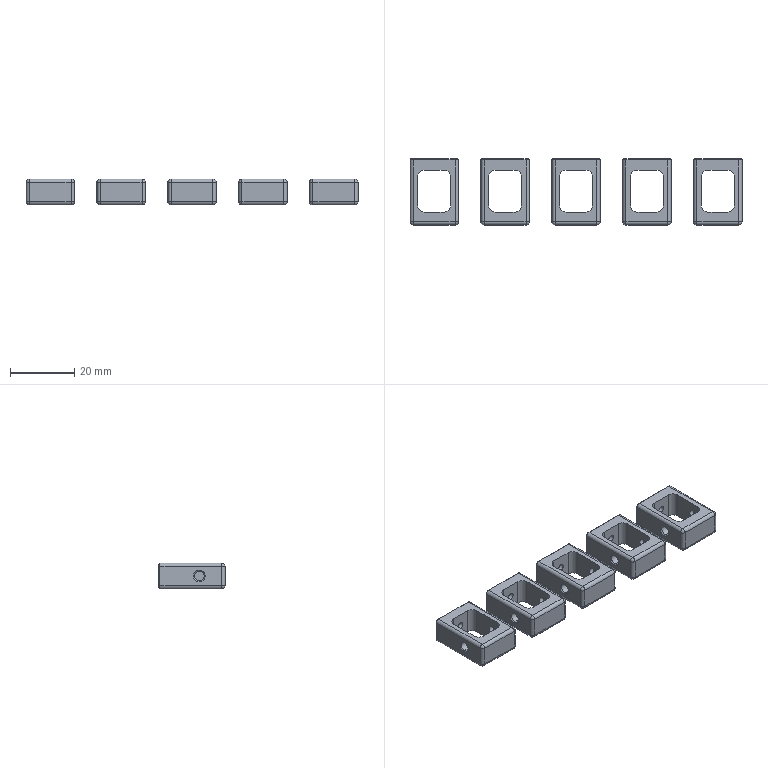NC program | NX | posted with a generic post | part box 103 x 20.5 x 8 mm
Lines 8374 to 9732 of 9732:
(PLANAR_MILL_COPY , TOOL : D6A45)
N16728 T01 M6
N16730 G54
N16732 G17 G0 G90 X-47. Y1.52 S9500 M3
N16734 G43 Z30. H1
N16736 Z0.5
N16738 G94 G1 Z-1. F1250.
N16740 X-47.7 Y1.116
N16742 G3 X-48.2 Y0.25 R1.
N16744 G1 Y-4.25
N16746 G3 X-47.1 Y-5.35 R1.1
N16748 G1 X-40.9
N16750 G3 X-39.8 Y-4.25 R1.1
N16752 G1 Y4.75
N16754 G3 X-40.9 Y5.85 R1.1
N16756 G1 X-47.1
N16758 G3 X-48.2 Y4.75 R1.1
N16760 G1 Y0.25
N16762 G3 X-47.7 Y-0.616 R1.
N16764 G1 X-47. Y-1.02
N16766 Z0.5
N16768 G0 Z30.
N16770 X-25. Y1.52
N16772 Z0.5
N16774 G1 Z-1.
N16776 X-25.7 Y1.116
N16778 G3 X-26.2 Y0.25 R1.
N16780 G1 Y-4.25
N16782 G3 X-25.1 Y-5.35 R1.1
N16784 G1 X-18.9
N16786 G3 X-17.8 Y-4.25 R1.1
N16788 G1 Y4.75
N16790 G3 X-18.9 Y5.85 R1.1
N16792 G1 X-25.1
N16794 G3 X-26.2 Y4.75 R1.1
N16796 G1 Y0.25
N16798 G3 X-25.7 Y-0.616 R1.
N16800 G1 X-25. Y-1.02
N16802 Z0.5
N16804 G0 Z30.
N16806 X-3. Y1.52
N16808 Z0.5
N16810 G1 Z-1.
N16812 X-3.7 Y1.116
N16814 G3 X-4.2 Y0.25 R1.
N16816 G1 Y-4.25
N16818 G3 X-3.1 Y-5.35 R1.1
N16820 G1 X3.1
N16822 G3 X4.2 Y-4.25 R1.1
N16824 G1 Y4.75
N16826 G3 X3.1 Y5.85 R1.1
N16828 G1 X-3.1
N16830 G3 X-4.2 Y4.75 R1.1
N16832 G1 Y0.25
N16834 G3 X-3.7 Y-0.616 R1.
N16836 G1 X-3. Y-1.02
N16838 Z0.5
N16840 G0 Z30.
N16842 X19. Y1.52
N16844 Z0.5
N16846 G1 Z-1.
N16848 X18.3 Y1.116
N16850 G3 X17.8 Y0.25 R1.
N16852 G1 Y-4.25
N16854 G3 X18.9 Y-5.35 R1.1
N16856 G1 X25.1
N16858 G3 X26.2 Y-4.25 R1.1
N16860 G1 Y4.75
N16862 G3 X25.1 Y5.85 R1.1
N16864 G1 X18.9
N16866 G3 X17.8 Y4.75 R1.1
N16868 G1 Y0.25
N16870 G3 X18.3 Y-0.616 R1.
N16872 G1 X19. Y-1.02
N16874 Z0.5
N16876 G0 Z30.
N16878 X47.
N16880 Z0.5
N16882 G1 Z-1.
N16884 X47.7 Y-0.616
N16886 G3 X48.2 Y0.25 R1.
N16888 G1 Y4.75
N16890 G3 X47.1 Y5.85 R1.1
N16892 G1 X40.9
N16894 G3 X39.8 Y4.75 R1.1
N16896 G1 Y-4.25
N16898 G3 X40.9 Y-5.35 R1.1
N16900 G1 X47.1
N16902 G3 X48.2 Y-4.25 R1.1
N16904 G1 Y0.25
N16906 G3 X47.7 Y1.116 R1.
N16908 G1 X47. Y1.52
N16910 Z0.5
N16912 G0 Z30.
N16914 M5
(ZLEVEL_PROFILE_1 , TOOL : D4R0.5)
N16916 T16 M6
N16918 G54
N16920 G17 G0 G90 X-35.174 Y12.738 S9500 M3
N16922 G43 Z30. H16
N16924 Z1.488
N16926 G94 G1 Z-0.012 F3000.
N16928 X-35.682 Y12.485
N16930 G3 X-35.903 Y12.152 R0.4
N16932 X-35.813 Y9.95 R10.813
N16934 G1 Y-9.25
N16936 G2 X-37.5 Y-10.937 R1.687
N16938 G1 X-50.5
N16940 G2 X-52.187 Y-9.25 R1.687
N16942 G1 Y9.95
N16944 X-52.109 Y10.153
N16946 X-52.09 Y12.155
N16948 X-52.133 Y12.154 Z-0.018
N16950 X-52.161 Y12.153 Z-0.024
N16952 X-52.25 Y10.153
N16954 X-52.27 Y9.95
N16956 Y-9.25
N16958 G3 X-50.5 Y-11.02 R1.77
N16960 G1 X-37.5
N16962 G3 X-35.73 Y-9.25 R1.77
N16964 G1 Y9.95
N16966 G2 X-35.826 Y12.151 R9.258
N16968 G1 X-35.785 Y12.152 Z-0.032
N16970 X-35.752 Y12.153 Z-0.039
N16972 G3 X-35.66 Y9.95 R7.979
N16974 G1 Y-9.25
N16976 G2 X-37.5 Y-11.09 R1.84
N16978 G1 X-50.5
N16980 G2 X-52.34 Y-9.25 R1.84
N16982 G1 Y9.95
N16984 X-52.223 Y12.151
N16986 X-52.264 Y12.15 Z-0.049
N16988 X-52.289 Z-0.058
N16990 X-52.299 Y11.846
N16992 X-52.414 Y9.95
N16994 Y-9.25
N16996 G3 X-50.5 Y-11.164 R1.914
N16998 G1 X-37.5
N17000 G3 X-35.586 Y-9.25 R1.914
N17002 G1 Y9.95
N17004 G2 X-35.684 Y12.151 R9.178
N17006 G1 X-35.643 Z-0.07
N17008 X-35.606 Y12.15 Z-0.083
N17010 G3 X-35.509 Y9.95 R11.176
N17012 G1 Y-9.25
N17014 G2 X-37.5 Y-11.241 R1.991
N17016 G1 X-50.5
N17018 G2 X-52.491 Y-9.25 R1.991
N17020 G1 Y9.95
N17022 X-52.473 Y10.153
N17024 X-52.354 Y12.15
N17026 X-52.406 Z-0.097
N17028 X-52.431 Z-0.112
N17030 G2 X-52.568 Y9.95 R21.926
N17032 G1 Y-9.25
N17034 G3 X-50.5 Y-11.318 R2.068
N17036 G1 X-37.5
N17038 G3 X-35.432 Y-9.25 R2.068
N17040 G1 Y9.95
N17042 G2 X-35.539 Y12.15 R11.662
N17044 G1 X-35.494 Z-0.129
N17046 X-35.463 Z-0.146
N17048 G3 X-35.355 Y9.95 R12.693
N17050 G1 Y-9.25
N17052 G2 X-37.5 Y-11.395 R2.145
N17054 G1 X-50.5
N17056 G2 X-52.645 Y-9.25 R2.145
N17058 G1 Y9.95
N17060 G3 X-52.522 Y12.15 R18.767
N17062 G1 X-52.574 Z-0.166
N17064 X-52.621 Y12.151 Z-0.186
N17066 G2 X-52.724 Y9.95 R19.723
N17068 G1 Y-9.25
N17070 G3 X-50.5 Y-11.474 R2.224
N17072 G1 X-37.5
N17074 G3 X-35.276 Y-9.25 R2.224
N17076 G1 Y9.95
N17078 G2 X-35.374 Y12.15 R17.072
N17080 G1 X-35.323 Z-0.21
N17082 X-35.286 Z-0.233
N17084 G3 X-35.197 Y9.95 R17.343
N17086 G1 Y-9.25
N17088 G2 X-37.5 Y-11.553 R2.303
N17090 G1 X-50.5
N17092 G2 X-52.803 Y-9.25 R2.303
N17094 G1 Y9.95
N17096 G3 X-52.716 Y12.151 R17.692
N17098 G1 X-52.761 Z-0.259
N17100 X-52.796 Y12.15 Z-0.286
N17102 G2 X-52.881 Y9.95 R18.852
N17104 G1 Y-9.25
N17106 G3 X-50.5 Y-11.631 R2.381
N17108 G1 X-37.5
N17110 G3 X-35.119 Y-9.25 R2.381
N17112 G1 Y9.95
N17114 G2 X-35.212 Y12.15 R17.769
N17116 G1 X-35.16 Z-0.315
N17118 X-35.13 Z-0.344
N17120 G3 X-35.044 Y9.95 R18.76
N17122 G1 Y-9.25
N17124 G2 X-37.5 Y-11.706 R2.456
N17126 G1 X-50.5
N17128 G2 X-52.956 Y-9.25 R2.456
N17130 G1 Y9.95
N17132 G3 X-52.877 Y12.15 R19.225
N17134 G1 X-52.92 Y12.151 Z-0.376
N17136 X-52.96 Z-0.408
N17138 G2 X-53.028 Y9.95 R23.684
N17140 G1 Y-9.25
N17142 G3 X-50.5 Y-11.778 R2.528
N17144 G1 X-37.5
N17146 G3 X-34.972 Y-9.25 R2.528
N17148 G1 Y9.95
N17150 G2 X-35.04 Y12.15 R23.709
N17152 G1 X-34.995 Y12.151 Z-0.443
N17154 X-34.96 Z-0.477
N17156 G3 X-34.903 Y9.95 R26.088
N17158 G1 Y-9.25
N17160 G2 X-37.5 Y-11.847 R2.597
N17162 G1 X-50.5
N17164 G2 X-53.097 Y-9.25 R2.597
N17166 G1 Y9.95
N17168 G3 X-53.04 Y12.152 R27.115
N17170 G1 X-53.073 Y12.151 Z-0.514
N17172 X-53.1 Y12.15 Z-0.551
N17174 G2 X-53.162 Y9.95 R24.243
N17176 G1 Y-9.25
N17178 G3 X-50.5 Y-11.912 R2.662
N17180 G1 X-37.5
N17182 G3 X-34.838 Y-9.25 R2.662
N17184 G1 Y9.95
N17186 G2 X-34.9 Y12.151 R24.274
N17188 G1 X-34.868 Z-0.59
N17190 X-34.841 Z-0.629
N17192 G3 X-34.779 Y9.95 R24.293
N17194 G1 Y-9.25
N17196 G2 X-37.5 Y-11.971 R2.721
N17198 G1 X-50.5
N17200 G2 X-53.221 Y-9.25 R2.721
N17202 G1 Y9.95
N17204 G3 X-53.159 Y12.151 R24.303
N17206 G1 X-53.193 Z-0.67
N17208 X-53.221 Y12.152 Z-0.711
N17210 G2 X-53.276 Y9.95 R30.814
N17212 G1 Y-9.25
N17214 G3 X-50.5 Y-12.026 R2.776
N17216 G1 X-37.5
N17218 G3 X-34.724 Y-9.25 R2.776
N17220 G1 Y9.95
N17222 G2 X-34.779 Y12.15 R30.37
N17224 G1 X-34.746 Y12.151 Z-0.754
N17226 X-34.728 Z-0.797
N17228 G3 X-34.675 Y9.95 R31.84
N17230 G1 Y-9.25
N17232 G2 X-37.5 Y-12.075 R2.825
N17234 G1 X-50.5
N17236 G2 X-53.325 Y-9.25 R2.825
N17238 G1 Y9.95
N17240 G3 X-53.274 Y12.151 R28.165
N17242 G1 X-53.299 Z-0.842
N17244 X-53.317 Z-0.887
N17246 G2 X-53.369 Y9.95 R25.497
N17248 G1 Y-9.25
N17250 G3 X-50.5 Y-12.119 R2.869
N17252 G1 X-37.5
N17254 G3 X-34.631 Y-9.25 R2.869
N17256 G1 Y9.95
N17258 G2 X-34.688 Y12.153 R33.716
N17260 G1 X-34.663 Y12.155 Z-0.933
N17262 X-34.647 Y12.156 Z-0.979
N17264 G3 X-34.593 Y9.95 R49.451
N17266 G1 Y-9.25
N17268 G2 X-37.5 Y-12.157 R2.907
N17270 G1 X-50.5
N17272 G2 X-53.407 Y-9.25 R2.907
N17274 G1 Y9.95
N17276 G3 X-53.362 Y12.15 R27.233
N17278 G1 X-53.384 Z-1.026
N17280 X-53.403 Z-1.074
N17282 G2 X-53.438 Y9.95 R31.796
N17284 G1 Y-9.25
N17286 G3 X-50.5 Y-12.188 R2.938
N17288 G1 X-37.5
N17290 G3 X-34.562 Y-9.25 R2.938
N17292 G1 Y9.95
N17294 G2 X-34.608 Y12.158 R55.585
N17296 G1 X-34.589 Y12.16 Z-1.122
N17298 X-34.572 Y12.161 Z-1.17
N17300 G3 X-34.537 Y9.95 R85.134
N17302 G1 Y-9.25
N17304 G2 X-37.5 Y-12.213 R2.963
N17306 G1 X-50.5
N17308 G2 X-53.463 Y-9.25 R2.963
N17310 G1 Y9.95
N17312 G3 X-53.436 Y12.152 R39.114
N17314 G1 X-53.446 Y12.153 Z-1.212
N17316 X-53.456 Z-1.253
N17318 X-53.458 Y10.717
N17320 X-53.469 Y10.435
N17322 G2 X-53.479 Y9.95 R3.288
N17324 G1 Y-9.25
N17326 G3 X-50.5 Y-12.229 R2.979
N17328 G1 X-37.5
N17330 G3 X-34.521 Y-9.25 R2.979
N17332 G1 Y9.95
N17334 G2 X-34.55 Y12.162 R76.351
N17336 G1 X-34.538 Y12.163 Z-1.294
N17338 X-34.531 Z-1.335
N17340 X-34.516 Y10.153
N17342 X-34.509 Y9.95
N17344 Y-9.25
N17346 G2 X-37.5 Y-12.241 R2.991
N17348 G1 X-50.5
N17350 G2 X-53.491 Y-9.25 R2.991
N17352 G1 Y9.95
N17354 G3 X-53.475 Y10.717 R24.677
N17356 G1 X-53.473 Y12.154
N17358 X-53.483 Y12.155 Z-1.376
N17360 X-53.49 Y12.156 Z-1.418
N17362 X-53.492 Y12.128
N17364 X-53.496 Y-9.273
N17366 G3 X-53.481 Y-9.57 R2.775
N17368 X-51.216 Y-12.161 R2.998
N17370 X-50.51 Y-12.248 R2.956
N17372 G1 X-37.5
N17374 G3 X-34.502 Y-9.25 R2.998
N17376 G1 Y9.95
N17378 X-34.511 Y12.165
N17380 X-34.505 Y12.162 Z-1.5
N17382 X-34.5 Y-9.247
N17384 G2 X-35.313 Y-11.3 R2.999
N17386 X-36.133 Y-11.918 R2.897
N17388 X-37.29 Y-12.241 R3.11
N17390 G1 X-37.49 Y-12.248
N17392 X-50.507
N17394 G2 X-51.524 Y-12.069 R2.963
N17396 X-53.453 Y-9.783 R3.012
N17398 G1 X-53.449
N17400 G2 X-53.498 Y-9.26 R3.149
N17402 G1 X-53.495 Y12.155
N17404 G3 X-53.695 Y12.502 R0.4
N17406 G1 X-54.218 Y12.804
N17408 Z0.
N17410 G0 Z3.
N17412 X-13.176 Y12.751
N17414 Z1.488
N17416 G1 Z-0.012
N17418 X-13.687 Y12.489
N17420 G3 X-13.905 Y12.153 R0.4
N17422 X-13.813 Y9.95 R11.978
N17424 G1 Y-9.25
N17426 G2 X-15.5 Y-10.937 R1.687
N17428 G1 X-28.5
N17430 G2 X-30.187 Y-9.25 R1.687
N17432 G1 Y9.95
N17434 X-30.114 Y10.153
N17436 X-30.103 Y12.155
N17438 X-30.16 Y12.153 Z-0.024
N17440 X-30.17 Y11.846
N17442 X-30.27 Y9.95
N17444 Y-9.25
N17446 G3 X-28.5 Y-11.02 R1.77
N17448 G1 X-15.5
N17450 G3 X-13.73 Y-9.25 R1.77
N17452 G1 Y9.95
N17454 G2 X-13.828 Y12.15 R10.515
N17456 G1 X-13.781 Z-0.032
N17458 X-13.776 Z-0.039
N17460 G3 X-13.66 Y9.95 R9.336
N17462 G1 Y-9.25
N17464 G2 X-15.5 Y-11.09 R1.84
N17466 G1 X-28.5
N17468 G2 X-30.34 Y-9.25 R1.84
N17470 G1 Y9.95
N17472 G3 X-30.226 Y12.15 R18.109
N17474 G1 X-30.26 Z-0.049
N17476 X-30.281 Z-0.058
N17478 G2 X-30.414 Y9.95 R19.419
N17480 G1 Y-9.25
N17482 G3 X-28.5 Y-11.164 R1.914
N17484 G1 X-15.5
N17486 G3 X-13.586 Y-9.25 R1.914
N17488 G1 Y9.95
N17490 G2 X-13.706 Y12.15 R9.374
N17492 G1 X-13.643 Z-0.07
N17494 X-13.618 Z-0.083
N17496 G3 X-13.509 Y9.95 R10.828
N17498 G1 Y-9.25
N17500 G2 X-15.5 Y-11.241 R1.991
N17502 G1 X-28.5
N17504 G2 X-30.491 Y-9.25 R1.991
N17506 G1 Y9.95
N17508 G3 X-30.349 Y12.15 R18.798
N17510 G1 X-30.406 Z-0.097
N17512 X-30.431 Z-0.112
N17514 G2 X-30.568 Y9.95 R19.096
N17516 G1 Y-9.25
N17518 G3 X-28.5 Y-11.318 R2.068
N17520 G1 X-15.5
N17522 G3 X-13.432 Y-9.25 R2.068
N17524 G1 Y9.95
N17526 G2 X-13.533 Y12.15 R11.751
N17528 G1 X-13.494 Z-0.129
N17530 X-13.46 Z-0.146
N17532 G3 X-13.355 Y9.95 R12.417
N17534 G1 Y-9.25
N17536 G2 X-15.5 Y-11.395 R2.145
N17538 G1 X-28.5
N17540 G2 X-30.645 Y-9.25 R2.145
N17542 G1 Y9.95
N17544 G3 X-30.525 Y12.15 R18.309
N17546 G1 X-30.574 Y12.151 Z-0.166
N17548 X-30.621 Z-0.186
N17550 G2 X-30.724 Y9.95 R18.599
N17552 G1 Y-9.25
N17554 G3 X-28.5 Y-11.474 R2.224
N17556 G1 X-15.5
N17558 G3 X-13.276 Y-9.25 R2.224
N17560 G1 Y9.95
N17562 G2 X-13.375 Y12.15 R15.774
N17564 G1 X-13.324 Z-0.21
N17566 X-13.276 Z-0.233
N17568 G3 X-13.197 Y9.95 R18.579
N17570 G1 Y-9.25
N17572 G2 X-15.5 Y-11.553 R2.303
N17574 G1 X-28.5
N17576 G2 X-30.803 Y-9.25 R2.303
N17578 G1 Y9.95
N17580 G3 X-30.711 Y12.151 R19.024
N17582 G1 X-30.767 Y12.15 Z-0.259
N17584 X-30.801 Z-0.286
N17586 G2 X-30.881 Y9.95 R18.564
N17588 G1 Y-9.25
N17590 G3 X-28.5 Y-11.631 R2.381
N17592 G1 X-15.5
N17594 G3 X-13.119 Y-9.25 R2.381
N17596 G1 Y9.95
N17598 G2 X-13.206 Y12.15 R16.93
N17600 G1 X-13.159 Z-0.315
N17602 X-13.128 Z-0.344
N17604 G3 X-13.044 Y9.95 R17.802
N17606 G1 Y-9.25
N17608 G2 X-15.5 Y-11.706 R2.456
N17610 G1 X-28.5
N17612 G2 X-30.956 Y-9.25 R2.456
N17614 G1 Y9.95
N17616 G3 X-30.877 Y12.15 R17.906
N17618 G1 X-30.92 Y12.151 Z-0.376
N17620 X-30.96 Z-0.408
N17622 G2 X-31.028 Y9.95 R19.425
N17624 G1 Y-9.25
N17626 G3 X-28.5 Y-11.778 R2.528
N17628 G1 X-15.5
N17630 G3 X-12.972 Y-9.25 R2.528
N17632 G1 Y9.95
N17634 G2 X-13.042 Y12.15 R23.333
N17636 G1 X-12.995 Z-0.443
N17638 X-12.967 Z-0.477
N17640 G3 X-12.903 Y9.95 R24.397
N17642 G1 Y-9.25
N17644 G2 X-15.5 Y-11.847 R2.597
N17646 G1 X-28.5
N17648 G2 X-31.097 Y-9.25 R2.597
N17650 G1 Y9.95
N17652 G3 X-31.037 Y12.15 R22.861
N17654 G1 X-31.069 Z-0.514
N17656 X-31.1 Z-0.551
N17658 G2 X-31.162 Y9.95 R24.207
N17660 G1 Y-9.25
N17662 G3 X-28.5 Y-11.912 R2.662
N17664 G1 X-15.5
N17666 G3 X-12.838 Y-9.25 R2.662
N17668 G1 Y9.95
N17670 G2 X-12.904 Y12.15 R23.42
N17672 G1 X-12.868 Y12.151 Z-0.59
N17674 X-12.841 Z-0.629
N17676 G3 X-12.779 Y9.95 R23.43
N17678 G1 Y-9.25
N17680 G2 X-15.5 Y-11.971 R2.721
N17682 G1 X-28.5
N17684 G2 X-31.221 Y-9.25 R2.721
N17686 G1 Y9.95
N17688 G3 X-31.16 Y12.151 R24.729
N17690 G1 X-31.193 Z-0.67
N17692 X-31.222 Z-0.711
N17694 G2 X-31.276 Y9.95 R29.092
N17696 G1 Y-9.25
N17698 G3 X-28.5 Y-12.026 R2.776
N17700 G1 X-15.5
N17702 G3 X-12.724 Y-9.25 R2.776
N17704 G1 Y9.95
N17706 G2 X-12.784 Y12.15 R25.622
N17708 G1 X-12.745 Z-0.754
N17710 X-12.726 Z-0.797
N17712 G3 X-12.675 Y9.95 R32.986
N17714 G1 Y-9.25
N17716 G2 X-15.5 Y-12.075 R2.825
N17718 G1 X-28.5
N17720 G2 X-31.325 Y-9.25 R2.825
N17722 G1 Y9.95
N17724 G3 X-31.275 Y12.152 R33.248
N17726 G1 X-31.299 Y12.151 Z-0.842
N17728 X-31.319 Z-0.887
N17730 G2 X-31.369 Y9.95 R28.16
N17732 G1 Y-9.25
N17734 G3 X-28.5 Y-12.119 R2.869
N17736 G1 X-15.5
N17738 G3 X-12.631 Y-9.25 R2.869
N17740 G1 Y9.95
N17742 G2 X-12.684 Y12.152 R32.786
N17744 G1 X-12.663 Y12.153 Z-0.933
N17746 X-12.645 Y12.154 Z-0.979
N17748 G3 X-12.593 Y9.95 R43.797
N17750 G1 Y-9.25
N17752 G2 X-15.5 Y-12.157 R2.907
N17754 G1 X-28.5
N17756 G2 X-31.407 Y-9.25 R2.907
N17758 G1 Y9.95
N17760 G3 X-31.363 Y12.15 R27.185
N17762 G1 X-31.386 Y12.152 Z-1.026
N17764 X-31.401 Y12.153 Z-1.074
N17766 G2 X-31.438 Y9.95 R32.305
N17768 G1 Y-9.25
N17770 G3 X-28.5 Y-12.188 R2.938
N17772 G1 X-15.5
N17774 G3 X-12.562 Y-9.25 R2.938
N17776 G1 Y9.95
N17778 G2 X-12.606 Y12.157 R59.474
N17780 G1 X-12.589 Y12.158 Z-1.122
N17782 X-12.572 Y12.159 Z-1.17
N17784 G3 X-12.537 Y9.95 R87.828
N17786 G1 Y-9.25
N17788 G2 X-15.5 Y-12.213 R2.963
N17790 G1 X-28.5
N17792 G2 X-31.463 Y-9.25 R2.963
N17794 G1 Y9.95
N17796 G3 X-31.436 Y12.155 R40.13
N17798 G1 X-31.446 Z-1.212
N17800 X-31.461 Y12.156 Z-1.253
N17802 G2 X-31.479 Y9.95 R52.452
N17804 G1 Y-9.25
N17806 G3 X-28.5 Y-12.229 R2.979
N17808 G1 X-15.5
N17810 G3 X-12.521 Y-9.25 R2.979
N17812 G1 Y9.95
N17814 G2 X-12.548 Y12.159 R75.91
N17816 G1 X-12.538 Y12.16 Z-1.294
N17818 X-12.53 Y12.161 Z-1.335
N17820 X-12.516 Y10.153
N17822 X-12.509 Y9.95
N17824 Y-9.25
N17826 G2 X-15.5 Y-12.241 R2.991
N17828 G1 X-28.5
N17830 G2 X-31.491 Y-9.25 R2.991
N17832 G1 Y9.95
N17834 G3 X-31.476 Y12.157 R76.85
N17836 G1 X-31.48 Z-1.376
N17838 X-31.491 Y12.158 Z-1.418
N17840 X-31.494 Y10.153
N17842 X-31.497 Y-9.272
N17844 G3 X-31.481 Y-9.57 R2.786
N17846 X-29.946 Y-11.876 R2.998
N17848 G1 X-29.717 Y-11.99
N17850 G3 X-29.082 Y-12.191 R2.998
N17852 X-28.5 Y-12.248 R2.998
N17854 G1 X-15.471
N17856 G3 X-13.606 Y-11.574 R2.998
N17858 G1 X-13.402 Y-11.391
N17860 G3 X-12.502 Y-9.25 R2.998
N17862 G1 Y9.95
N17864 X-12.511 Y12.162
N17866 X-12.505 Y12.16 Z-1.5
N17868 X-12.5 Y-9.247
N17870 G2 X-13.605 Y-11.572 R2.999
N17872 X-14.078 Y-11.889 R2.738
N17874 X-15.35 Y-12.242 R2.945
N17876 G1 X-15.49 Y-12.248
N17878 X-28.5
N17880 G2 X-29.496 Y-12.076 R2.942
N17882 G1 X-29.761 Y-11.972
N17884 G2 X-31.133 Y-10.683 R3.033
N17886 X-31.45 Y-9.783 R2.954
N17888 X-31.498 Y-9.26 R3.379
N17890 G1 X-31.496 Y12.128
N17892 X-31.495 Y12.157
N17894 G3 X-31.676 Y12.514 R0.4
N17896 G1 X-32.206 Y12.859
N17898 Z0.
N17900 G0 Z3.
N17902 X8.825 Y12.741
N17904 Z1.488
N17906 G1 Z-0.012
N17908 X8.323 Y12.489
N17910 G3 X8.103 Y12.154 R0.4
N17912 X8.187 Y9.95 R11.509
N17914 G1 Y-9.25
N17916 G2 X6.5 Y-10.937 R1.687
N17918 G1 X-6.5
N17920 G2 X-8.187 Y-9.25 R1.687
N17922 G1 Y9.95
N17924 X-8.168 Y10.153
N17926 X-8.095 Y12.155
N17928 X-8.134 Y12.153 Z-0.018
N17930 X-8.159 Y12.152 Z-0.024
N17932 X-8.237 Y10.153
N17934 X-8.27 Y9.95
N17936 Y-9.25
N17938 G3 X-6.5 Y-11.02 R1.77
N17940 G1 X6.5
N17942 G3 X8.27 Y-9.25 R1.77
N17944 G1 Y9.95
N17946 G2 X8.179 Y12.151 R11.718
N17948 G1 X8.221 Y12.15 Z-0.032
N17950 X8.232 Z-0.039
N17952 G3 X8.34 Y9.95 R10.746
N17954 G1 Y-9.25
N17956 G2 X6.5 Y-11.09 R1.84
N17958 G1 X-6.5
N17960 G2 X-8.34 Y-9.25 R1.84
N17962 G1 Y9.95
N17964 X-8.298 Y10.153
N17966 X-8.216 Y12.15
N17968 X-8.26 Z-0.049
N17970 X-8.274 Z-0.058
N17972 X-8.285 Y11.846
N17974 X-8.378 Y10.153
N17976 X-8.414 Y9.95
N17978 Y-9.25
N17980 G3 X-6.5 Y-11.164 R1.914
N17982 G1 X6.5
N17984 G3 X8.414 Y-9.25 R1.914
N17986 G1 Y9.95
N17988 G2 X8.294 Y12.15 R9.95
N17990 G1 X8.357 Z-0.07
N17992 X8.372 Z-0.083
N17994 G3 X8.491 Y9.95 R10.072
N17996 G1 Y-9.25
N17998 G2 X6.5 Y-11.241 R1.991
N18000 G1 X-6.5
N18002 G2 X-8.491 Y-9.25 R1.991
N18004 G1 Y9.95
N18006 G3 X-8.348 Y12.15 R19.167
N18008 G1 X-8.405 Z-0.097
N18010 X-8.435 Z-0.112
N18012 G2 X-8.568 Y9.95 R20.551
N18014 G1 Y-9.25
N18016 G3 X-6.5 Y-11.318 R2.068
N18018 G1 X6.5
N18020 G3 X8.568 Y-9.25 R2.068
N18022 G1 Y9.95
N18024 G2 X8.465 Y12.15 R10.922
N18026 G1 X8.506 Z-0.129
N18028 X8.538 Z-0.146
N18030 G3 X8.645 Y9.95 R11.832
N18032 G1 Y-9.25
N18034 G2 X6.5 Y-11.395 R2.145
N18036 G1 X-6.5
N18038 G2 X-8.645 Y-9.25 R2.145
N18040 G1 Y9.95
N18042 G3 X-8.521 Y12.15 R16.287
N18044 G1 X-8.574 Z-0.166
N18046 X-8.61 Z-0.186
N18048 G2 X-8.724 Y9.95 R17.188
N18050 G1 Y-9.25
N18052 G3 X-6.5 Y-11.474 R2.224
N18054 G1 X6.5
N18056 G3 X8.724 Y-9.25 R2.224
N18058 G1 Y9.95
N18060 G2 X8.621 Y12.15 R13.891
N18062 G1 X8.677 Z-0.21
N18064 X8.716 Z-0.233
N18066 G3 X8.803 Y9.95 R20.219
N18068 G1 Y-9.25
N18070 G2 X6.5 Y-11.553 R2.303
N18072 G1 X-6.5
N18074 G2 X-8.803 Y-9.25 R2.303
N18076 G1 Y9.95
N18078 G3 X-8.712 Y12.15 R22.154
N18080 G1 X-8.76 Z-0.259
N18082 X-8.798 Z-0.286
N18084 G2 X-8.881 Y9.95 R17.875
N18086 G1 Y-9.25
N18088 G3 X-6.5 Y-11.631 R2.381
N18090 G1 X6.5
N18092 G3 X8.881 Y-9.25 R2.381
N18094 G1 Y9.95
N18096 G2 X8.798 Y12.15 R17.875
N18098 G1 X8.841 Z-0.315
N18100 X8.872 Z-0.344
N18102 G3 X8.956 Y9.95 R17.78
N18104 G1 Y-9.25
N18106 G2 X6.5 Y-11.706 R2.456
N18108 G1 X-6.5
N18110 G2 X-8.956 Y-9.25 R2.456
N18112 G1 Y9.95
N18114 G3 X-8.872 Y12.15 R17.78
N18116 G1 X-8.92 Z-0.376
N18118 X-8.953 Z-0.408
N18120 G2 X-9.028 Y9.95 R21.292
N18122 G1 Y-9.25
N18124 G3 X-6.5 Y-11.778 R2.528
N18126 G1 X6.5
N18128 G3 X9.028 Y-9.25 R2.528
N18130 G1 Y9.95
N18132 G2 X8.953 Y12.15 R21.292
N18134 G1 X8.998 Z-0.443
N18136 X9.041 Z-0.477
N18138 G3 X9.097 Y9.95 R25.737
N18140 G1 Y-9.25
N18142 G2 X6.5 Y-11.847 R2.597
N18144 G1 X-6.5
N18146 G2 X-9.097 Y-9.25 R2.597
N18148 G1 Y9.95
N18150 G3 X-9.041 Y12.15 R25.737
N18152 G1 X-9.073 Z-0.514
N18154 X-9.098 Z-0.551
N18156 G2 X-9.162 Y9.95 R23.081
N18158 G1 Y-9.25
N18160 G3 X-6.5 Y-11.912 R2.662
N18162 G1 X6.5
N18164 G3 X9.162 Y-9.25 R2.662
N18166 G1 Y9.95
N18168 G2 X9.098 Y12.15 R23.084
N18170 G1 X9.132 Y12.151 Z-0.59
N18172 X9.16 Z-0.629
N18174 G3 X9.221 Y9.95 R24.413
N18176 G1 Y-9.25
N18178 G2 X6.5 Y-11.971 R2.721
N18180 G1 X-6.5
N18182 G2 X-9.221 Y-9.25 R2.721
N18184 G1 Y9.95
N18186 G3 X-9.16 Y12.151 R24.402
N18188 G1 X-9.193 Z-0.67
N18190 X-9.222 Z-0.711
N18192 G2 X-9.276 Y9.95 R30.188
N18194 G1 Y-9.25
N18196 G3 X-6.5 Y-12.026 R2.776
N18198 G1 X6.5
N18200 G3 X9.276 Y-9.25 R2.776
N18202 G1 Y9.95
N18204 G2 X9.222 Y12.152 R30.24
N18206 G1 X9.249 Y12.151 Z-0.754
N18208 X9.273 Z-0.797
N18210 G3 X9.325 Y9.95 R32.017
N18212 G1 Y-9.25
N18214 G2 X6.5 Y-12.075 R2.825
N18216 G1 X-6.5
N18218 G2 X-9.325 Y-9.25 R2.825
N18220 G1 Y9.95
N18222 G3 X-9.275 Y12.151 R29.563
N18224 G1 X-9.3 Y12.15 Z-0.842
N18226 X-9.32 Z-0.887
N18228 G2 X-9.369 Y9.95 R27.833
N18230 G1 Y-9.25
N18232 G3 X-6.5 Y-12.119 R2.869
N18234 G1 X6.5
N18236 G3 X9.369 Y-9.25 R2.869
N18238 G1 Y9.95
N18240 G2 X9.316 Y12.15 R33.813
N18242 G1 X9.337 Y12.151 Z-0.933
N18244 X9.354 Y12.152 Z-0.979
N18246 G3 X9.407 Y9.95 R41.05
N18248 G1 Y-9.25
N18250 G2 X6.5 Y-12.157 R2.907
N18252 G1 X-6.5
N18254 G2 X-9.407 Y-9.25 R2.907
N18256 G1 Y9.95
N18258 G3 X-9.362 Y12.152 R27.311
N18260 G1 X-9.383 Y12.154 Z-1.026
N18262 X-9.405 Y12.156 Z-1.074
N18264 G2 X-9.438 Y9.95 R32.12
N18266 G1 Y-9.25
N18268 G3 X-6.5 Y-12.188 R2.938
N18270 G1 X6.5
N18272 G3 X9.438 Y-9.25 R2.938
N18274 G1 Y9.95
N18276 G2 X9.393 Y12.155 R76.635
N18278 G1 X9.411 Y12.156 Z-1.122
N18280 X9.428 Y12.157 Z-1.17
N18282 G3 X9.463 Y9.95 R98.832
N18284 G1 Y-9.25
N18286 G2 X6.5 Y-12.213 R2.963
N18288 G1 X-6.5
N18290 G2 X-9.463 Y-9.25 R2.963
N18292 G1 Y9.95
N18294 G3 X-9.436 Y12.157 R39.697
N18296 G1 X-9.446 Z-1.212
N18298 X-9.458 Z-1.253
N18300 X-9.457 Y11.846
N18302 X-9.468 Y10.153
N18304 X-9.479 Y9.95
N18306 Y-9.25
N18308 G3 X-6.5 Y-12.229 R2.979
N18310 G1 X6.5
N18312 G3 X9.479 Y-9.25 R2.979
N18314 G1 Y9.95
N18316 X9.47 Y10.153
N18318 X9.454 Y12.158
N18320 X9.462 Y12.159 Z-1.294
N18322 X9.472 Z-1.335
N18324 X9.482 Y10.153
N18326 X9.491 Y9.95
N18328 Y-9.25
N18330 G2 X6.5 Y-12.241 R2.991
N18332 G1 X-6.5
N18334 G2 X-9.491 Y-9.25 R2.991
N18336 G1 Y9.95
N18338 X-9.48 Y10.153
N18340 X-9.474 Y12.159
N18342 X-9.482 Z-1.376
N18344 X-9.49 Y12.16 Z-1.418
N18346 X-9.492 Y12.128
N18348 X-9.493 Y10.153
N18350 X-9.498 Y9.95
N18352 Y-9.25
N18354 G3 X-6.5 Y-12.248 R2.998
N18356 G1 X6.5
N18358 G3 X9.498 Y-9.25 R2.998
N18360 G1 Y9.95
N18362 X9.49 Y12.16
N18364 X9.495 Y12.158 Z-1.5
N18366 X9.497 Y-9.324
N18368 G2 X8.387 Y-11.579 R2.989
N18370 G1 X8.386 Y-11.582
N18372 X8.087 Y-11.809
N18374 X7.668 Y-12.011
N18376 X7.593 Y-12.041
N18378 G2 X6.55 Y-12.247 R2.987
N18380 G1 X6.498 Y-12.248
N18382 X-6.503
N18384 X-6.562 Y-12.247
N18386 G2 X-7.939 Y-11.88 R3.007
N18388 X-8.737 Y-11.246 R2.745
N18390 X-9.464 Y-9.697 R2.999
N18392 X-9.498 Y-9.25 R2.991
N18394 G1 X-9.495 Y12.159
N18396 G3 X-9.695 Y12.506 R0.4
N18398 G1 X-10.219 Y12.809
N18400 Z0.
N18402 G0 Z3.
N18404 X30.813 Y12.797
N18406 Z1.488
N18408 G1 Z-0.012
N18410 X30.306 Y12.502
N18412 G3 X30.107 Y12.155 R0.4
N18414 G1 X30.114 Y10.153
N18416 X30.187 Y9.95
N18418 Y-9.25
N18420 G2 X28.5 Y-10.937 R1.687
N18422 G1 X15.5
N18424 G2 X13.813 Y-9.25 R1.687
N18426 G1 Y9.95
N18428 X13.913 Y12.155
N18430 X13.863 Y12.152 Z-0.018
N18432 X13.837 Y12.15 Z-0.024
N18434 X13.773 Y10.153
N18436 X13.73 Y9.95
N18438 Y-9.25
N18440 G3 X15.5 Y-11.02 R1.77
N18442 G1 X28.5
N18444 G3 X30.27 Y-9.25 R1.77
N18446 G1 Y9.95
N18448 G2 X30.178 Y12.152 R12.211
N18450 G1 X30.221 Y12.151 Z-0.032
N18452 X30.247 Y12.15 Z-0.039
N18454 G3 X30.34 Y9.95 R11.494
N18456 G1 Y-9.25
N18458 G2 X28.5 Y-11.09 R1.84
N18460 G1 X15.5
N18462 G2 X13.66 Y-9.25 R1.84
N18464 G1 Y9.95
N18466 X13.705 Y10.153
N18468 X13.79 Y12.15
N18470 X13.735 Z-0.049
N18472 X13.727 Z-0.058
N18474 G2 X13.586 Y9.95 R19.404
N18476 G1 Y-9.25
N18478 G3 X15.5 Y-11.164 R1.914
N18480 G1 X28.5
N18482 G3 X30.414 Y-9.25 R1.914
N18484 G1 Y9.95
N18486 G2 X30.313 Y12.151 R10.075
N18488 G1 X30.357 Z-0.07
N18490 X30.389 Z-0.083
N18492 G3 X30.491 Y9.95 R9.024
N18494 G1 Y-9.25
N18496 G2 X28.5 Y-11.241 R1.991
N18498 G1 X15.5
N18500 G2 X13.509 Y-9.25 R1.991
N18502 G1 Y9.95
N18504 X13.526 Y10.153
N18506 X13.647 Y12.15
N18508 X13.596 Z-0.097
N18510 X13.555 Z-0.112
N18512 G2 X13.432 Y9.95 R17.545
N18514 G1 Y-9.25
N18516 G3 X15.5 Y-11.318 R2.068
N18518 G1 X28.5
N18520 G3 X30.568 Y-9.25 R2.068
N18522 G1 Y9.95
N18524 G2 X30.461 Y12.15 R10.15
N18526 G1 X30.507 Z-0.129
N18528 X30.538 Z-0.146
N18530 G3 X30.645 Y9.95 R12.907
N18532 G1 Y-9.25
N18534 G2 X28.5 Y-11.395 R2.145
N18536 G1 X15.5
N18538 G2 X13.355 Y-9.25 R2.145
N18540 G1 Y9.95
N18542 G3 X13.476 Y12.15 R16.428
N18544 G1 X13.426 Z-0.166
N18546 X13.383 Z-0.186
N18548 G2 X13.276 Y9.95 R18.66
N18550 G1 Y-9.25
N18552 G3 X15.5 Y-11.474 R2.224
N18554 G1 X28.5
N18556 G3 X30.724 Y-9.25 R2.224
N18558 G1 Y9.95
N18560 G2 X30.616 Y12.15 R19.048
N18562 G1 X30.678 Z-0.21
N18564 X30.705 Z-0.233
N18566 G3 X30.803 Y9.95 R20.973
N18568 G1 Y-9.25
N18570 G2 X28.5 Y-11.553 R2.303
N18572 G1 X15.5
N18574 G2 X13.197 Y-9.25 R2.303
N18576 G1 Y9.95
N18578 G3 X13.276 Y12.15 R18.579
N18580 G1 X13.238 Z-0.259
N18582 X13.206 Z-0.286
N18584 G2 X13.119 Y9.95 R16.93
N18586 G1 Y-9.25
N18588 G3 X15.5 Y-11.631 R2.381
N18590 G1 X28.5
N18592 G3 X30.881 Y-9.25 R2.381
N18594 G1 Y9.95
N18596 G2 X30.801 Y12.15 R18.564
N18598 G1 X30.841 Z-0.315
N18600 X30.877 Z-0.344
N18602 G3 X30.956 Y9.95 R17.906
N18604 G1 Y-9.25
N18606 G2 X28.5 Y-11.706 R2.456
N18608 G1 X15.5
N18610 G2 X13.044 Y-9.25 R2.456
N18612 G1 Y9.95
N18614 G3 X13.128 Y12.15 R17.802
N18616 G1 X13.08 Z-0.376
N18618 X13.042 Z-0.408
N18620 G2 X12.972 Y9.95 R23.333
N18622 G1 Y-9.25
N18624 G3 X15.5 Y-11.778 R2.528
N18626 G1 X28.5
N18628 G3 X31.028 Y-9.25 R2.528
N18630 G1 Y9.95
N18632 G2 X30.96 Y12.151 R19.425
N18634 G1 X30.999 Z-0.443
N18636 X31.037 Y12.15 Z-0.477
N18638 G3 X31.097 Y9.95 R22.861
N18640 G1 Y-9.25
N18642 G2 X28.5 Y-11.847 R2.597
N18644 G1 X15.5
N18646 G2 X12.903 Y-9.25 R2.597
N18648 G1 Y9.95
N18650 G3 X12.967 Y12.15 R24.397
N18652 G1 X12.927 Z-0.514
N18654 X12.904 Z-0.551
N18656 G2 X12.838 Y9.95 R23.42
N18658 G1 Y-9.25
N18660 G3 X15.5 Y-11.912 R2.662
N18662 G1 X28.5
N18664 G3 X31.162 Y-9.25 R2.662
N18666 G1 Y9.95
N18668 G2 X31.1 Y12.15 R24.209
N18670 G1 X31.132 Y12.151 Z-0.59
N18672 X31.16 Z-0.629
N18674 G3 X31.221 Y9.95 R24.736
N18676 G1 Y-9.25
N18678 G2 X28.5 Y-11.971 R2.721
N18680 G1 X15.5
N18682 G2 X12.779 Y-9.25 R2.721
N18684 G1 Y9.95
N18686 G3 X12.841 Y12.151 R23.43
N18688 G1 X12.807 Y12.15 Z-0.67
N18690 X12.784 Z-0.711
N18692 G2 X12.724 Y9.95 R25.622
N18694 G1 Y-9.25
N18696 G3 X15.5 Y-12.026 R2.776
N18698 G1 X28.5
N18700 G3 X31.276 Y-9.25 R2.776
N18702 G1 Y9.95
N18704 G2 X31.222 Y12.152 R29.106
N18706 G1 X31.248 Z-0.754
N18708 X31.275 Z-0.797
N18710 G3 X31.325 Y9.95 R33.53
N18712 G1 Y-9.25
N18714 G2 X28.5 Y-12.075 R2.825
N18716 G1 X15.5
N18718 G2 X12.675 Y-9.25 R2.825
N18720 G1 Y9.95
N18722 G3 X12.726 Y12.15 R32.804
N18724 G1 X12.7 Y12.151 Z-0.842
N18726 X12.68 Y12.152 Z-0.887
N18728 G2 X12.631 Y9.95 R27.974
N18730 G1 Y-9.25
N18732 G3 X15.5 Y-12.119 R2.869
N18734 G1 X28.5
N18736 G3 X31.369 Y-9.25 R2.869
N18738 G1 Y9.95
N18740 G2 X31.316 Y12.151 R34.661
N18742 G1 X31.337 Y12.15 Z-0.933
N18744 X31.355 Z-0.979
N18746 G3 X31.407 Y9.95 R42.325
N18748 G1 Y-9.25
N18750 G2 X28.5 Y-12.157 R2.907
N18752 G1 X15.5
N18754 G2 X12.593 Y-9.25 R2.907
N18756 G1 Y9.95
N18758 G3 X12.637 Y12.155 R28.211
N18760 G1 X12.616 Y12.156 Z-1.026
N18762 X12.597 Z-1.074
N18764 G2 X12.562 Y9.95 R32.34
N18766 G1 Y-9.25
N18768 G3 X15.5 Y-12.188 R2.938
N18770 G1 X28.5
N18772 G3 X31.438 Y-9.25 R2.938
N18774 G1 Y9.95
N18776 G2 X31.392 Y12.152 R56.529
N18778 G1 X31.411 Y12.153 Z-1.122
N18780 X31.428 Y12.154 Z-1.17
N18782 G3 X31.463 Y9.95 R90.183
N18784 G1 Y-9.25
N18786 G2 X28.5 Y-12.213 R2.963
N18788 G1 X15.5
N18790 G2 X12.537 Y-9.25 R2.963
N18792 G1 Y9.95
N18794 G3 X12.565 Y12.159 R39.861
N18796 G1 X12.554 Z-1.212
N18798 X12.545 Z-1.253
N18800 X12.542 Y10.717
N18802 X12.531 Y10.435
N18804 G2 X12.521 Y9.95 R3.235
N18806 G1 Y-9.25
N18808 G3 X15.5 Y-12.229 R2.979
N18810 G1 X28.5
N18812 G3 X31.479 Y-9.25 R2.979
N18814 G1 Y9.95
N18816 X31.471 Y10.153
N18818 X31.462 Y10.999
N18820 X31.455 Y11.995
N18822 X31.448 Y12.155
N18824 X31.462 Y12.156 Z-1.294
N18826 X31.469 Y12.157 Z-1.335
N18828 X31.476 Y11.282
N18830 X31.483 Y10.153
N18832 X31.491 Y9.95
N18834 Y-9.25
N18836 G2 X28.5 Y-12.241 R2.991
N18838 G1 X15.5
N18840 G2 X12.509 Y-9.25 R2.991
N18842 G1 Y9.95
N18844 G3 X12.525 Y10.717 R24.766
N18846 G1 X12.527 Y12.161
N18848 X12.519 Y12.162 Z-1.376
N18850 X12.51 Z-1.418
N18852 X12.508 Y12.128
N18854 X12.507 Y10.153
N18856 X12.502 Y9.95
N18858 Y-9.25
N18860 G3 X15.5 Y-12.248 R2.998
N18862 G1 X28.5
N18864 G3 X31.498 Y-9.287 R2.998
N18866 G1 Y-9.25
N18868 Y9.95
N18870 X31.495 Y10.153
N18872 X31.491 Y12.128
N18874 X31.489 Y12.158
N18876 X31.495 Y12.157 Z-1.5
N18878 X31.498 Y-9.287
N18880 G2 X30.701 Y-11.283 R2.968
N18882 G1 X30.702 Y-11.284
N18884 X30.689 Y-11.299
N18886 X30.397 Y-11.574
N18888 G2 X29.689 Y-12.005 R3.359
N18890 X29.047 Y-12.197 R2.852
N18892 X28.5 Y-12.248 R3.232
N18894 G1 X15.49
N18896 X15.449 Y-12.247
N18898 G2 X14.06 Y-11.879 R3.103
N18900 X13.588 Y-11.559 R2.811
N18902 X12.891 Y-10.731 R3.118
N18904 G1 X12.723 Y-10.379
N18906 X12.692 Y-10.3
N18908 G2 X12.533 Y-9.679 R3.09
N18910 X12.502 Y-9.263 R2.836
N18912 G1 X12.505 Y12.161
N18914 G3 X12.305 Y12.507 R0.4
N18916 G1 X11.783 Y12.809
N18918 Z0.
N18920 G0 Z3.
N18922 X52.79 Y12.831
N18924 Z1.488
N18926 G1 Z-0.012
N18928 X52.25 Y12.501
N18930 G3 X52.059 Y12.15 R0.4
N18932 G1 X52.109 Y10.153
N18934 X52.187 Y9.95
N18936 Y-9.25
N18938 G2 X50.5 Y-10.937 R1.687
N18940 G1 X37.5
N18942 G2 X35.813 Y-9.25 R1.687
N18944 G1 Y9.95
N18946 X35.849 Y10.153
N18948 X35.907 Y11.846
N18950 X35.91 Y12.153
N18952 X35.863 Y12.151 Z-0.018
N18954 X35.845 Y12.15 Z-0.024
N18956 X35.781 Y10.153
N18958 X35.73 Y9.95
N18960 Y-9.25
N18962 G3 X37.5 Y-11.02 R1.77
N18964 G1 X50.5
N18966 G3 X52.27 Y-9.25 R1.77
N18968 G1 Y9.95
N18970 G2 X52.145 Y12.15 R14.513
N18972 G1 X52.215 Z-0.032
N18974 X52.243 Z-0.039
N18976 G3 X52.34 Y9.95 R11.799
N18978 G1 Y-9.25
N18980 G2 X50.5 Y-11.09 R1.84
N18982 G1 X37.5
N18984 G2 X35.66 Y-9.25 R1.84
N18986 G1 Y9.95
N18988 X35.703 Y10.153
N18990 X35.794 Y12.15
N18992 X35.74 Z-0.049
N18994 X35.727 Z-0.058
N18996 G2 X35.586 Y9.95 R25.754
N18998 G1 Y-9.25
N19000 G3 X37.5 Y-11.164 R1.914
N19002 G1 X50.5
N19004 G3 X52.414 Y-9.25 R1.914
N19006 G1 Y9.95
N19008 G2 X52.316 Y12.15 R10.975
N19010 G1 X52.357 Y12.151 Z-0.07
N19012 X52.394 Y12.152 Z-0.083
N19014 G3 X52.491 Y9.95 R10.031
N19016 G1 Y-9.25
N19018 G2 X50.5 Y-11.241 R1.991
N19020 G1 X37.5
N19022 G2 X35.509 Y-9.25 R1.991
N19024 G1 Y9.95
N19026 G3 X35.642 Y12.15 R24.332
N19028 G1 X35.595 Z-0.097
N19030 X35.558 Z-0.112
N19032 G2 X35.432 Y9.95 R16.369
N19034 G1 Y-9.25
N19036 G3 X37.5 Y-11.318 R2.068
N19038 G1 X50.5
N19040 G3 X52.568 Y-9.25 R2.068
N19042 G1 Y9.95
N19044 G2 X52.463 Y12.151 R10.22
N19046 G1 X52.507 Y12.15 Z-0.129
N19048 X52.541 Z-0.146
N19050 G3 X52.645 Y9.95 R12.053
N19052 G1 Y-9.25
N19054 G2 X50.5 Y-11.395 R2.145
N19056 G1 X37.5
N19058 G2 X35.355 Y-9.25 R2.145
N19060 G1 Y9.95
N19062 G3 X35.476 Y12.15 R15.899
N19064 G1 X35.426 Z-0.166
N19066 X35.38 Z-0.186
N19068 G2 X35.276 Y9.95 R18.924
N19070 G1 Y-9.25
N19072 G3 X37.5 Y-11.474 R2.224
N19074 G1 X50.5
N19076 G3 X52.724 Y-9.25 R2.224
N19078 G1 Y9.95
N19080 G2 X52.627 Y12.151 R16.637
N19082 G1 X52.677 Z-0.21
N19084 X52.716 Z-0.233
N19086 G3 X52.803 Y9.95 R17.677
N19088 G1 Y-9.25
N19090 G2 X50.5 Y-11.553 R2.303
N19092 G1 X37.5
N19094 G2 X35.197 Y-9.25 R2.303
N19096 G1 Y9.95
N19098 G3 X35.286 Y12.15 R17.35
N19100 G1 X35.238 Z-0.259
N19102 X35.212 Z-0.286
N19104 G2 X35.119 Y9.95 R17.769
N19106 G1 Y-9.25
N19108 G3 X37.5 Y-11.631 R2.381
N19110 G1 X50.5
N19112 G3 X52.881 Y-9.25 R2.381
N19114 G1 Y9.95
N19116 G2 X52.796 Y12.15 R18.849
N19118 G1 X52.841 Z-0.315
N19120 X52.877 Z-0.344
N19122 G3 X52.956 Y9.95 R19.225
N19124 G1 Y-9.25
N19126 G2 X50.5 Y-11.706 R2.456
N19128 G1 X37.5
N19130 G2 X35.044 Y-9.25 R2.456
N19132 G1 Y9.95
N19134 G3 X35.13 Y12.15 R18.76
N19136 G1 X35.08 Z-0.376
N19138 X35.04 Z-0.408
N19140 G2 X34.972 Y9.95 R23.709
N19142 G1 Y-9.25
N19144 G3 X37.5 Y-11.778 R2.528
N19146 G1 X50.5
N19148 G3 X53.028 Y-9.25 R2.528
N19150 G1 Y9.95
N19152 G2 X52.96 Y12.151 R23.684
N19154 G1 X52.999 Z-0.443
N19156 X53.04 Y12.152 Z-0.477
N19158 G3 X53.097 Y9.95 R26.941
N19160 G1 Y-9.25
N19162 G2 X50.5 Y-11.847 R2.597
N19164 G1 X37.5
N19166 G2 X34.903 Y-9.25 R2.597
N19168 G1 Y9.95
N19170 G3 X34.96 Y12.151 R26.088
N19172 G1 X34.93 Z-0.514
N19174 X34.9 Z-0.551
N19176 G2 X34.838 Y9.95 R24.274
N19178 G1 Y-9.25
N19180 G3 X37.5 Y-11.912 R2.662
N19182 G1 X50.5
N19184 G3 X53.162 Y-9.25 R2.662
N19186 G1 Y9.95
N19188 G2 X53.1 Y12.15 R24.243
N19190 G1 X53.132 Z-0.59
N19192 X53.159 Y12.151 Z-0.629
N19194 G3 X53.221 Y9.95 R24.309
N19196 G1 Y-9.25
N19198 G2 X50.5 Y-11.971 R2.721
N19200 G1 X37.5
N19202 G2 X34.779 Y-9.25 R2.721
N19204 G1 Y9.95
N19206 G3 X34.841 Y12.151 R24.293
N19208 G1 X34.807 Y12.15 Z-0.67
N19210 X34.779 Z-0.711
N19212 G2 X34.724 Y9.95 R30.37
N19214 G1 Y-9.25
N19216 G3 X37.5 Y-12.026 R2.776
N19218 G1 X50.5
N19220 G3 X53.276 Y-9.25 R2.776
N19222 G1 Y9.95
N19224 G2 X53.221 Y12.152 R30.832
N19226 G1 X53.249 Z-0.754
N19228 X53.272 Y12.151 Z-0.797
N19230 G3 X53.325 Y9.95 R30.716
N19232 G1 Y-9.25
N19234 G2 X50.5 Y-12.075 R2.825
N19236 G1 X37.5
N19238 G2 X34.675 Y-9.25 R2.825
N19240 G1 Y9.95
N19242 G3 X34.726 Y12.151 R29.111
N19244 G1 X34.701 Y12.153 Z-0.842
N19246 X34.682 Y12.154 Z-0.887
N19248 G2 X34.631 Y9.95 R25.64
N19250 G1 Y-9.25
N19252 G3 X37.5 Y-12.119 R2.869
N19254 G1 X50.5
N19256 G3 X53.369 Y-9.25 R2.869
N19258 G1 Y9.95
N19260 G2 X53.312 Y12.151 R32.482
N19262 G1 X53.337 Z-0.933
N19264 X53.353 Z-0.979
N19266 G3 X53.407 Y9.95 R44.733
N19268 G1 Y-9.25
N19270 G2 X50.5 Y-12.157 R2.907
N19272 G1 X37.5
N19274 G2 X34.593 Y-9.25 R2.907
N19276 G1 Y9.95
N19278 G3 X34.638 Y12.157 R27.476
N19280 G1 X34.616 Y12.158 Z-1.026
N19282 X34.6 Y12.159 Z-1.074
N19284 G2 X34.562 Y9.95 R31.
N19286 G1 Y-9.25
N19288 G3 X37.5 Y-12.188 R2.938
N19290 G1 X50.5
N19292 G3 X53.438 Y-9.25 R2.938
N19294 G1 Y9.95
N19296 G2 X53.395 Y12.15 R54.144
N19298 G1 X53.413 Y12.151 Z-1.122
N19300 X53.428 Y12.152 Z-1.17
N19302 G3 X53.463 Y9.95 R83.256
N19304 G1 Y-9.25
N19306 G2 X50.5 Y-12.213 R2.963
N19308 G1 X37.5
N19310 G2 X34.537 Y-9.25 R2.963
N19312 G1 Y9.95
N19314 G3 X34.564 Y12.161 R40.729
N19316 G1 X34.554 Y12.164 Z-1.212
N19318 X34.541 Y12.167 Z-1.253
N19320 G2 X34.521 Y9.95 R43.821
N19322 G1 Y-9.25
N19324 G3 X37.5 Y-12.229 R2.979
N19326 G1 X50.5
N19328 G3 X53.479 Y-9.25 R2.979
N19330 G1 Y9.95
N19332 X53.468 Y10.153
N19334 X53.452 Y12.153
N19336 X53.462 Y12.154 Z-1.294
N19338 X53.471 Z-1.335
N19340 X53.481 Y10.153
N19342 X53.491 Y9.95
N19344 Y-9.25
N19346 G2 X50.5 Y-12.241 R2.991
N19348 G1 X37.5
N19350 G2 X34.509 Y-9.25 R2.991
N19352 G1 Y9.95
N19354 X34.518 Y10.153
N19356 X34.528 Y11.846
N19358 X34.525 Y12.167
N19360 X34.518 Y12.166 Z-1.376
N19362 X34.51 Y12.165 Z-1.418
N19364 X34.507 Y10.153
N19366 X34.502 Y9.95
N19368 Y-9.25
N19370 G3 X37.5 Y-12.248 R2.998
N19372 G1 X50.5
N19374 G3 X53.498 Y-9.287 R2.998
N19376 G1 Y-9.25
N19378 Y9.95
N19380 X53.49 Y12.156
N19382 X53.495 Y12.155 Z-1.5
N19384 X53.498 Y-9.287
N19386 G2 X52.392 Y-11.575 R2.987
N19388 G1 X52.386 Y-11.582
N19390 X52.075 Y-11.816
N19392 G2 X51.315 Y-12.135 R4.006
N19394 X50.851 Y-12.227 R2.683
N19396 G1 Y-12.226
N19398 X50.568 Y-12.246
N19400 X50.51 Y-12.248
N19402 X37.49
N19404 X37.44 Y-12.247
N19406 G2 X36.06 Y-11.879 R3.08
N19408 X35.191 Y-11.152 R2.814
N19410 X34.877 Y-10.7 R2.554
N19412 G1 X34.72 Y-10.372
N19414 X34.701 Y-10.324
N19416 G2 X34.533 Y-9.679 R3.063
N19418 X34.502 Y-9.258 R2.886
N19420 G1 X34.505 Y12.163
N19422 G3 X34.305 Y12.509 R0.4
N19424 G1 X33.783 Y12.811
N19426 Z0.
N19428 G0 Z30.
N19430 M5
N19432 M2